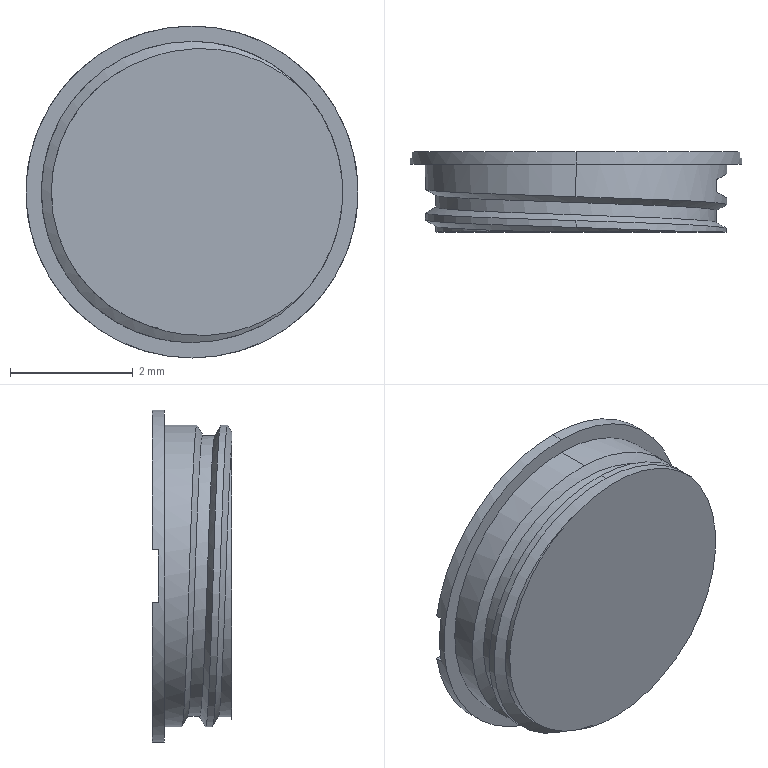Part | SolidWorks | features ICE 3, Extrusion 1, Helix 1, SweepCut 1 | 1 solid | 19 faces | box 5.4 x 1.3 x 5.4 mm | volume 23.765 mm3 | plane 10 | cylinder 6 | spline 3 | commonest cylinder face diameters 4.9 x4 5.4 x2
STEP:
#1=CARTESIAN_POINT('',(0.,1.3,2.7));
#2=VERTEX_POINT('',#1);
#3=CARTESIAN_POINT('',(2.666,1.3,0.425));
#4=VERTEX_POINT('',#3);
#5=CARTESIAN_POINT('',(0.,1.3,0.));
#6=DIRECTION('',(0.,1.,0.));
#7=DIRECTION('',(0.,0.,1.));
#8=AXIS2_PLACEMENT_3D('',#5,#6,#7);
#9=CIRCLE('',#8,2.7);
#10=EDGE_CURVE('',#2,#4,#9,.T.);
#11=ORIENTED_EDGE('',*,*,#10,.F.);
#12=CARTESIAN_POINT('',(0.,1.1,2.7));
#13=VERTEX_POINT('',#12);
#14=CARTESIAN_POINT('',(0.,1.3,2.7));
#15=DIRECTION('',(0.,-1.,0.));
#16=VECTOR('',#15,1000.);
#17=LINE('',#14,#16);
#18=EDGE_CURVE('',#2,#13,#17,.T.);
#19=ORIENTED_EDGE('',*,*,#18,.T.);
#20=CARTESIAN_POINT('',(0.,1.1,-2.7));
#21=VERTEX_POINT('',#20);
#22=CARTESIAN_POINT('',(0.,1.1,0.));
#23=DIRECTION('',(0.,-1.,0.));
#24=DIRECTION('',(0.,0.,-1.));
#25=AXIS2_PLACEMENT_3D('',#22,#23,#24);
#26=CIRCLE('',#25,2.7);
#27=EDGE_CURVE('',#21,#13,#26,.T.);
#28=ORIENTED_EDGE('',*,*,#27,.F.);
#29=CARTESIAN_POINT('',(0.,1.3,-2.7));
#30=VERTEX_POINT('',#29);
#31=CARTESIAN_POINT('',(0.,1.3,-2.7));
#32=DIRECTION('',(0.,-1.,0.));
#33=VECTOR('',#32,1000.);
#34=LINE('',#31,#33);
#35=EDGE_CURVE('',#30,#21,#34,.T.);
#36=ORIENTED_EDGE('',*,*,#35,.F.);
#37=CARTESIAN_POINT('',(2.666,1.3,-0.425));
#38=VERTEX_POINT('',#37);
#39=CARTESIAN_POINT('',(0.,1.3,0.));
#40=DIRECTION('',(0.,1.,0.));
#41=DIRECTION('',(0.,0.,1.));
#42=AXIS2_PLACEMENT_3D('',#39,#40,#41);
#43=CIRCLE('',#42,2.7);
#44=EDGE_CURVE('',#38,#30,#43,.T.);
#45=ORIENTED_EDGE('',*,*,#44,.F.);
#46=CARTESIAN_POINT('',(2.666,1.2,-0.425));
#47=VERTEX_POINT('',#46);
#48=CARTESIAN_POINT('',(2.666,1.3,-0.425));
#49=DIRECTION('',(0.,-1.,0.));
#50=VECTOR('',#49,1000.);
#51=LINE('',#48,#50);
#52=EDGE_CURVE('',#38,#47,#51,.T.);
#53=ORIENTED_EDGE('',*,*,#52,.T.);
#54=CARTESIAN_POINT('',(2.666,1.2,0.425));
#55=VERTEX_POINT('',#54);
#56=CARTESIAN_POINT('',(0.,1.2,0.));
#57=DIRECTION('',(0.,-1.,0.));
#58=DIRECTION('',(0.,0.,-1.));
#59=AXIS2_PLACEMENT_3D('',#56,#57,#58);
#60=CIRCLE('',#59,2.7);
#61=EDGE_CURVE('',#47,#55,#60,.T.);
#62=ORIENTED_EDGE('',*,*,#61,.T.);
#63=CARTESIAN_POINT('',(2.666,1.3,0.425));
#64=DIRECTION('',(0.,1.,0.));
#65=VECTOR('',#64,1000.);
#66=LINE('',#63,#65);
#67=EDGE_CURVE('',#55,#4,#66,.T.);
#68=ORIENTED_EDGE('',*,*,#67,.T.);
#69=EDGE_LOOP('',(#11,#19,#28,#36,#45,#53,#62,#68));
#70=FACE_OUTER_BOUND('',#69,.T.);
#71=CARTESIAN_POINT('',(0.,1.3,0.));
#72=DIRECTION('',(0.,-1.,0.));
#73=DIRECTION('',(0.,0.,-1.));
#74=AXIS2_PLACEMENT_3D('',#71,#72,#73);
#75=CYLINDRICAL_SURFACE('',#74,2.7);
#76=ADVANCED_FACE('',(#70),#75,.T.);
#77=CARTESIAN_POINT('',(0.,1.1,-2.45));
#78=VERTEX_POINT('',#77);
#79=CARTESIAN_POINT('',(0.,1.1,2.45));
#80=VERTEX_POINT('',#79);
#81=CARTESIAN_POINT('',(0.,1.1,0.));
#82=DIRECTION('',(0.,-1.,0.));
#83=DIRECTION('',(0.,0.,-1.));
#84=AXIS2_PLACEMENT_3D('',#81,#82,#83);
#85=CIRCLE('',#84,2.45);
#86=EDGE_CURVE('',#78,#80,#85,.T.);
#87=ORIENTED_EDGE('',*,*,#86,.T.);
#88=CARTESIAN_POINT('',(0.,0.5692,2.45));
#89=VERTEX_POINT('',#88);
#90=CARTESIAN_POINT('',(0.,1.1,2.45));
#91=DIRECTION('',(0.,-1.,0.));
#92=VECTOR('',#91,1000.);
#93=LINE('',#90,#92);
#94=EDGE_CURVE('',#80,#89,#93,.T.);
#95=ORIENTED_EDGE('',*,*,#94,.T.);
#96=CARTESIAN_POINT('',(0.,0.3192,-2.45));
#97=VERTEX_POINT('',#96);
#98=CARTESIAN_POINT('',(0.,0.3192,-2.45));
#99=CARTESIAN_POINT('',(0.6565,0.3416,-2.45));
#100=CARTESIAN_POINT('',(1.225,0.3609,-2.122));
#101=CARTESIAN_POINT('',(2.45,0.4026,-1.415));
#102=CARTESIAN_POINT('',(2.45,0.4442,0.));
#103=CARTESIAN_POINT('',(2.45,0.4859,1.415));
#104=CARTESIAN_POINT('',(1.225,0.5276,2.122));
#105=CARTESIAN_POINT('',(0.6565,0.5469,2.45));
#106=CARTESIAN_POINT('',(0.,0.5692,2.45));
#107=(BOUNDED_CURVE()B_SPLINE_CURVE(2,(#98,#99,#100,#101,#102,#103,#104,#105,#106),.UNSPECIFIED.,.F.,.F.)B_SPLINE_CURVE_WITH_KNOTS((3,2,2,2,3),(0.4167,0.4444,0.5,0.5556,0.5833),.UNSPECIFIED.)CURVE()GEOMETRIC_REPRESENTATION_ITEM()RATIONAL_B_SPLINE_CURVE((0.933,0.933,1.,0.866,1.,0.866,1.,0.933,0.933))REPRESENTATION_ITEM(''));
#108=EDGE_CURVE('',#97,#89,#107,.T.);
#109=ORIENTED_EDGE('',*,*,#108,.F.);
#110=CARTESIAN_POINT('',(0.,0.4308,-2.45));
#111=VERTEX_POINT('',#110);
#112=CARTESIAN_POINT('',(0.,1.1,-2.45));
#113=DIRECTION('',(0.,-1.,0.));
#114=VECTOR('',#113,1000.);
#115=LINE('',#112,#114);
#116=EDGE_CURVE('',#111,#97,#115,.T.);
#117=ORIENTED_EDGE('',*,*,#116,.F.);
#118=CARTESIAN_POINT('',(2.45,0.5558,0.));
#119=VERTEX_POINT('',#118);
#120=CARTESIAN_POINT('',(0.,0.4308,-2.45));
#121=CARTESIAN_POINT('',(0.6565,0.4531,-2.45));
#122=CARTESIAN_POINT('',(1.225,0.4724,-2.122));
#123=CARTESIAN_POINT('',(2.45,0.5141,-1.415));
#124=CARTESIAN_POINT('',(2.45,0.5558,0.));
#125=(BOUNDED_CURVE()B_SPLINE_CURVE(2,(#120,#121,#122,#123,#124),.UNSPECIFIED.,.F.,.F.)B_SPLINE_CURVE_WITH_KNOTS((3,2,3),(0.75,0.7778,0.8333),.UNSPECIFIED.)CURVE()GEOMETRIC_REPRESENTATION_ITEM()RATIONAL_B_SPLINE_CURVE((0.933,0.933,1.,0.866,1.))REPRESENTATION_ITEM(''));
#126=EDGE_CURVE('',#111,#119,#125,.T.);
#127=ORIENTED_EDGE('',*,*,#126,.T.);
#128=CARTESIAN_POINT('',(2.287,0.65,0.8792));
#129=VERTEX_POINT('',#128);
#130=CARTESIAN_POINT('',(2.287,0.65,0.8792));
#131=CARTESIAN_POINT('',(2.395,0.5875,0.5979));
#132=CARTESIAN_POINT('',(2.45,0.5558,0.3015));
#133=CARTESIAN_POINT('',(2.45,0.5558,0.));
#134=(BOUNDED_CURVE()B_SPLINE_CURVE(3,(#130,#131,#132,#133),.UNSPECIFIED.,.F.,.F.)B_SPLINE_CURVE_WITH_KNOTS((4,4),(5.916,6.283),.UNSPECIFIED.)CURVE()GEOMETRIC_REPRESENTATION_ITEM()RATIONAL_B_SPLINE_CURVE((1.,0.9888,0.9888,1.))REPRESENTATION_ITEM(''));
#135=EDGE_CURVE('',#129,#119,#134,.T.);
#136=ORIENTED_EDGE('',*,*,#135,.F.);
#137=CARTESIAN_POINT('',(2.287,0.85,0.8792));
#138=VERTEX_POINT('',#137);
#139=CARTESIAN_POINT('',(2.287,1.1,0.8792));
#140=DIRECTION('',(0.,-1.,0.));
#141=VECTOR('',#140,1000.);
#142=LINE('',#139,#141);
#143=EDGE_CURVE('',#138,#129,#142,.T.);
#144=ORIENTED_EDGE('',*,*,#143,.F.);
#145=CARTESIAN_POINT('',(2.45,0.9442,0.));
#146=VERTEX_POINT('',#145);
#147=CARTESIAN_POINT('',(2.45,0.9442,0.));
#148=CARTESIAN_POINT('',(2.45,0.9442,0.3015));
#149=CARTESIAN_POINT('',(2.395,0.9125,0.5979));
#150=CARTESIAN_POINT('',(2.287,0.85,0.8792));
#151=(BOUNDED_CURVE()B_SPLINE_CURVE(3,(#147,#148,#149,#150),.UNSPECIFIED.,.F.,.F.)B_SPLINE_CURVE_WITH_KNOTS((4,4),(3.142,3.509),.UNSPECIFIED.)CURVE()GEOMETRIC_REPRESENTATION_ITEM()RATIONAL_B_SPLINE_CURVE((1.,0.9888,0.9888,1.))REPRESENTATION_ITEM(''));
#152=EDGE_CURVE('',#146,#138,#151,.T.);
#153=ORIENTED_EDGE('',*,*,#152,.F.);
#154=CARTESIAN_POINT('',(0.,0.8192,-2.45));
#155=VERTEX_POINT('',#154);
#156=CARTESIAN_POINT('',(0.,0.8192,-2.45));
#157=CARTESIAN_POINT('',(0.6565,0.8416,-2.45));
#158=CARTESIAN_POINT('',(1.225,0.8609,-2.122));
#159=CARTESIAN_POINT('',(2.45,0.9026,-1.415));
#160=CARTESIAN_POINT('',(2.45,0.9442,0.));
#161=(BOUNDED_CURVE()B_SPLINE_CURVE(2,(#156,#157,#158,#159,#160),.UNSPECIFIED.,.F.,.F.)B_SPLINE_CURVE_WITH_KNOTS((3,2,3),(0.75,0.7778,0.8333),.UNSPECIFIED.)CURVE()GEOMETRIC_REPRESENTATION_ITEM()RATIONAL_B_SPLINE_CURVE((0.933,0.933,1.,0.866,1.))REPRESENTATION_ITEM(''));
#162=EDGE_CURVE('',#155,#146,#161,.T.);
#163=ORIENTED_EDGE('',*,*,#162,.F.);
#164=CARTESIAN_POINT('',(0.,1.1,-2.45));
#165=DIRECTION('',(0.,-1.,0.));
#166=VECTOR('',#165,1000.);
#167=LINE('',#164,#166);
#168=EDGE_CURVE('',#78,#155,#167,.T.);
#169=ORIENTED_EDGE('',*,*,#168,.F.);
#170=EDGE_LOOP('',(#87,#95,#109,#117,#127,#136,#144,#153,#163,#169));
#171=FACE_OUTER_BOUND('',#170,.T.);
#172=CARTESIAN_POINT('',(0.,1.1,0.));
#173=DIRECTION('',(0.,-1.,0.));
#174=DIRECTION('',(0.,0.,-1.));
#175=AXIS2_PLACEMENT_3D('',#172,#173,#174);
#176=CYLINDRICAL_SURFACE('',#175,2.45);
#177=ADVANCED_FACE('',(#171),#176,.T.);
#178=CARTESIAN_POINT('',(1.884,0.,-1.566));
#179=VERTEX_POINT('',#178);
#180=CARTESIAN_POINT('',(0.,0.1808,2.45));
#181=VERTEX_POINT('',#180);
#182=CARTESIAN_POINT('',(1.884,0.,-1.566));
#183=CARTESIAN_POINT('',(2.45,0.02969,-0.8856));
#184=CARTESIAN_POINT('',(2.45,0.05577,0.));
#185=CARTESIAN_POINT('',(2.45,0.09744,1.415));
#186=CARTESIAN_POINT('',(1.225,0.1391,2.122));
#187=CARTESIAN_POINT('',(0.6565,0.1584,2.45));
#188=CARTESIAN_POINT('',(0.,0.1808,2.45));
#189=(BOUNDED_CURVE()B_SPLINE_CURVE(2,(#182,#183,#184,#185,#186,#187,#188),.UNSPECIFIED.,.F.,.F.)B_SPLINE_CURVE_WITH_KNOTS((3,2,2,3),(0.4634,0.5,0.5556,0.5833),.UNSPECIFIED.)CURVE()GEOMETRIC_REPRESENTATION_ITEM()RATIONAL_B_SPLINE_CURVE((0.9398,0.9117,1.,0.866,1.,0.933,0.933))REPRESENTATION_ITEM(''));
#190=EDGE_CURVE('',#179,#181,#189,.T.);
#191=ORIENTED_EDGE('',*,*,#190,.T.);
#192=CARTESIAN_POINT('',(0.,0.06923,2.45));
#193=VERTEX_POINT('',#192);
#194=CARTESIAN_POINT('',(0.,1.1,2.45));
#195=DIRECTION('',(0.,-1.,0.));
#196=VECTOR('',#195,1000.);
#197=LINE('',#194,#196);
#198=EDGE_CURVE('',#181,#193,#197,.T.);
#199=ORIENTED_EDGE('',*,*,#198,.T.);
#200=CARTESIAN_POINT('',(1.884,0.,1.566));
#201=VERTEX_POINT('',#200);
#202=CARTESIAN_POINT('',(1.884,0.,1.566));
#203=CARTESIAN_POINT('',(1.604,0.01467,1.903));
#204=CARTESIAN_POINT('',(1.225,0.02756,2.122));
#205=CARTESIAN_POINT('',(0.6565,0.0469,2.45));
#206=CARTESIAN_POINT('',(0.,0.06923,2.45));
#207=(BOUNDED_CURVE()B_SPLINE_CURVE(2,(#202,#203,#204,#205,#206),.UNSPECIFIED.,.F.,.F.)B_SPLINE_CURVE_WITH_KNOTS((3,2,3),(0.2033,0.2222,0.25),.UNSPECIFIED.)CURVE()GEOMETRIC_REPRESENTATION_ITEM()RATIONAL_B_SPLINE_CURVE((0.9398,0.9543,1.,0.933,0.933))REPRESENTATION_ITEM(''));
#208=EDGE_CURVE('',#201,#193,#207,.T.);
#209=ORIENTED_EDGE('',*,*,#208,.F.);
#210=CARTESIAN_POINT('',(0.,0.,0.));
#211=DIRECTION('',(0.,-1.,0.));
#212=DIRECTION('',(0.,0.,-1.));
#213=AXIS2_PLACEMENT_3D('',#210,#211,#212);
#214=CIRCLE('',#213,2.45);
#215=EDGE_CURVE('',#179,#201,#214,.T.);
#216=ORIENTED_EDGE('',*,*,#215,.F.);
#217=EDGE_LOOP('',(#191,#199,#209,#216));
#218=FACE_OUTER_BOUND('',#217,.T.);
#219=CARTESIAN_POINT('',(0.,1.1,0.));
#220=DIRECTION('',(0.,-1.,0.));
#221=DIRECTION('',(0.,0.,-1.));
#222=AXIS2_PLACEMENT_3D('',#219,#220,#221);
#223=CYLINDRICAL_SURFACE('',#222,2.45);
#224=ADVANCED_FACE('',(#218),#223,.T.);
#225=ORIENTED_EDGE('',*,*,#198,.F.);
#226=CARTESIAN_POINT('',(0.,0.1808,2.45));
#227=CARTESIAN_POINT('',(-0.6565,0.2031,2.45));
#228=CARTESIAN_POINT('',(-1.225,0.2224,2.122));
#229=CARTESIAN_POINT('',(-2.45,0.2641,1.415));
#230=CARTESIAN_POINT('',(-2.45,0.3058,0.));
#231=CARTESIAN_POINT('',(-2.45,0.3474,-1.415));
#232=CARTESIAN_POINT('',(-1.225,0.3891,-2.122));
#233=CARTESIAN_POINT('',(-0.6565,0.4084,-2.45));
#234=CARTESIAN_POINT('',(0.,0.4308,-2.45));
#235=(BOUNDED_CURVE()B_SPLINE_CURVE(2,(#226,#227,#228,#229,#230,#231,#232,#233,#234),.UNSPECIFIED.,.F.,.F.)B_SPLINE_CURVE_WITH_KNOTS((3,2,2,2,3),(0.5833,0.6111,0.6667,0.7222,0.75),.UNSPECIFIED.)CURVE()GEOMETRIC_REPRESENTATION_ITEM()RATIONAL_B_SPLINE_CURVE((0.933,0.933,1.,0.866,1.,0.866,1.,0.933,0.933))REPRESENTATION_ITEM(''));
#236=EDGE_CURVE('',#181,#111,#235,.T.);
#237=ORIENTED_EDGE('',*,*,#236,.T.);
#238=ORIENTED_EDGE('',*,*,#116,.T.);
#239=CARTESIAN_POINT('',(0.,0.06923,2.45));
#240=CARTESIAN_POINT('',(-0.6565,0.09156,2.45));
#241=CARTESIAN_POINT('',(-1.225,0.1109,2.122));
#242=CARTESIAN_POINT('',(-2.45,0.1526,1.415));
#243=CARTESIAN_POINT('',(-2.45,0.1942,0.));
#244=CARTESIAN_POINT('',(-2.45,0.2359,-1.415));
#245=CARTESIAN_POINT('',(-1.225,0.2776,-2.122));
#246=CARTESIAN_POINT('',(-0.6565,0.2969,-2.45));
#247=CARTESIAN_POINT('',(0.,0.3192,-2.45));
#248=(BOUNDED_CURVE()B_SPLINE_CURVE(2,(#239,#240,#241,#242,#243,#244,#245,#246,#247),.UNSPECIFIED.,.F.,.F.)B_SPLINE_CURVE_WITH_KNOTS((3,2,2,2,3),(0.25,0.2778,0.3333,0.3889,0.4167),.UNSPECIFIED.)CURVE()GEOMETRIC_REPRESENTATION_ITEM()RATIONAL_B_SPLINE_CURVE((0.933,0.933,1.,0.866,1.,0.866,1.,0.933,0.933))REPRESENTATION_ITEM(''));
#249=EDGE_CURVE('',#193,#97,#248,.T.);
#250=ORIENTED_EDGE('',*,*,#249,.F.);
#251=EDGE_LOOP('',(#225,#237,#238,#250));
#252=FACE_OUTER_BOUND('',#251,.T.);
#253=CARTESIAN_POINT('',(0.,1.1,0.));
#254=DIRECTION('',(0.,-1.,0.));
#255=DIRECTION('',(0.,0.,-1.));
#256=AXIS2_PLACEMENT_3D('',#253,#254,#255);
#257=CYLINDRICAL_SURFACE('',#256,2.45);
#258=ADVANCED_FACE('',(#252),#257,.T.);
#259=CARTESIAN_POINT('',(-2.666,1.3,0.425));
#260=VERTEX_POINT('',#259);
#261=CARTESIAN_POINT('',(0.,1.3,0.425));
#262=DIRECTION('',(1.,0.,0.));
#263=VECTOR('',#262,1000.);
#264=LINE('',#261,#263);
#265=EDGE_CURVE('',#260,#4,#264,.T.);
#266=ORIENTED_EDGE('',*,*,#265,.F.);
#267=CARTESIAN_POINT('',(0.,1.3,0.));
#268=DIRECTION('',(0.,1.,0.));
#269=DIRECTION('',(0.,0.,1.));
#270=AXIS2_PLACEMENT_3D('',#267,#268,#269);
#271=CIRCLE('',#270,2.7);
#272=EDGE_CURVE('',#260,#2,#271,.T.);
#273=ORIENTED_EDGE('',*,*,#272,.T.);
#274=ORIENTED_EDGE('',*,*,#10,.T.);
#275=EDGE_LOOP('',(#266,#273,#274));
#276=FACE_OUTER_BOUND('',#275,.T.);
#277=CARTESIAN_POINT('',(0.,1.3,0.));
#278=DIRECTION('',(0.,1.,0.));
#279=DIRECTION('',(0.,0.,1.));
#280=AXIS2_PLACEMENT_3D('',#277,#278,#279);
#281=PLANE('',#280);
#282=ADVANCED_FACE('',(#276),#281,.T.);
#283=ORIENTED_EDGE('',*,*,#94,.F.);
#284=CARTESIAN_POINT('',(0.,1.1,0.));
#285=DIRECTION('',(0.,-1.,0.));
#286=DIRECTION('',(0.,0.,-1.));
#287=AXIS2_PLACEMENT_3D('',#284,#285,#286);
#288=CIRCLE('',#287,2.45);
#289=EDGE_CURVE('',#80,#78,#288,.T.);
#290=ORIENTED_EDGE('',*,*,#289,.T.);
#291=ORIENTED_EDGE('',*,*,#168,.T.);
#292=CARTESIAN_POINT('',(0.,0.5692,2.45));
#293=CARTESIAN_POINT('',(-0.6565,0.5916,2.45));
#294=CARTESIAN_POINT('',(-1.225,0.6109,2.122));
#295=CARTESIAN_POINT('',(-2.45,0.6526,1.415));
#296=CARTESIAN_POINT('',(-2.45,0.6942,0.));
#297=CARTESIAN_POINT('',(-2.45,0.7359,-1.415));
#298=CARTESIAN_POINT('',(-1.225,0.7776,-2.122));
#299=CARTESIAN_POINT('',(-0.6565,0.7969,-2.45));
#300=CARTESIAN_POINT('',(0.,0.8192,-2.45));
#301=(BOUNDED_CURVE()B_SPLINE_CURVE(2,(#292,#293,#294,#295,#296,#297,#298,#299,#300),.UNSPECIFIED.,.F.,.F.)B_SPLINE_CURVE_WITH_KNOTS((3,2,2,2,3),(0.5833,0.6111,0.6667,0.7222,0.75),.UNSPECIFIED.)CURVE()GEOMETRIC_REPRESENTATION_ITEM()RATIONAL_B_SPLINE_CURVE((0.933,0.933,1.,0.866,1.,0.866,1.,0.933,0.933))REPRESENTATION_ITEM(''));
#302=EDGE_CURVE('',#89,#155,#301,.T.);
#303=ORIENTED_EDGE('',*,*,#302,.F.);
#304=EDGE_LOOP('',(#283,#290,#291,#303));
#305=FACE_OUTER_BOUND('',#304,.T.);
#306=CARTESIAN_POINT('',(0.,1.1,0.));
#307=DIRECTION('',(0.,-1.,0.));
#308=DIRECTION('',(0.,0.,-1.));
#309=AXIS2_PLACEMENT_3D('',#306,#307,#308);
#310=CYLINDRICAL_SURFACE('',#309,2.45);
#311=ADVANCED_FACE('',(#305),#310,.T.);
#312=CARTESIAN_POINT('',(-0.686,0.,-2.181));
#313=VERTEX_POINT('',#312);
#314=CARTESIAN_POINT('',(1.884,0.,-1.566));
#315=CARTESIAN_POINT('',(1.723,0.,-1.738));
#316=CARTESIAN_POINT('',(1.538,0.,-1.887));
#317=CARTESIAN_POINT('',(1.138,0.,-2.124));
#318=CARTESIAN_POINT('',(0.9167,0.,-2.215));
#319=CARTESIAN_POINT('',(0.5773,0.,-2.297));
#320=CARTESIAN_POINT('',(0.4626,0.,-2.316));
#321=CARTESIAN_POINT('',(0.2298,0.,-2.336));
#322=CARTESIAN_POINT('',(0.111,0.,-2.337));
#323=CARTESIAN_POINT('',(-0.2385,0.,-2.315));
#324=CARTESIAN_POINT('',(-0.4654,0.,-2.266));
#325=CARTESIAN_POINT('',(-0.686,0.,-2.181));
#326=B_SPLINE_CURVE_WITH_KNOTS('',3,(#314,#315,#316,#317,#318,#319,#320,#321,#322,#323,#324,#325),.UNSPECIFIED.,.F.,.F.,(4,2,2,2,2,4),(0.0001717,0.0008766,0.001582,0.001934,0.002286,0.002991),.UNSPECIFIED.);
#327=EDGE_CURVE('',#179,#313,#326,.T.);
#328=ORIENTED_EDGE('',*,*,#327,.F.);
#329=ORIENTED_EDGE('',*,*,#215,.T.);
#330=CARTESIAN_POINT('',(-0.686,0.,2.181));
#331=VERTEX_POINT('',#330);
#332=CARTESIAN_POINT('',(-0.686,0.,2.181));
#333=CARTESIAN_POINT('',(-0.2463,0.,2.349));
#334=CARTESIAN_POINT('',(0.237,0.,2.38));
#335=CARTESIAN_POINT('',(1.149,0.,2.158));
#336=CARTESIAN_POINT('',(1.564,0.,1.908));
#337=CARTESIAN_POINT('',(1.884,0.,1.566));
#338=B_SPLINE_CURVE_WITH_KNOTS('',3,(#332,#333,#334,#335,#336,#337),.UNSPECIFIED.,.F.,.F.,(4,2,4),(0.,0.001406,0.002811),.UNSPECIFIED.);
#339=EDGE_CURVE('',#331,#201,#338,.T.);
#340=ORIENTED_EDGE('',*,*,#339,.F.);
#341=CARTESIAN_POINT('',(-0.686,0.,-2.181));
#342=CARTESIAN_POINT('',(-0.9183,0.,-2.108));
#343=CARTESIAN_POINT('',(-1.138,0.,-1.998));
#344=CARTESIAN_POINT('',(-1.528,0.,-1.718));
#345=CARTESIAN_POINT('',(-1.703,0.,-1.545));
#346=CARTESIAN_POINT('',(-1.916,0.,-1.254));
#347=CARTESIAN_POINT('',(-1.979,0.,-1.152));
#348=CARTESIAN_POINT('',(-2.09,0.,-0.937));
#349=CARTESIAN_POINT('',(-2.137,0.,-0.824));
#350=CARTESIAN_POINT('',(-2.211,0.,-0.5953));
#351=CARTESIAN_POINT('',(-2.239,0.,-0.4786));
#352=CARTESIAN_POINT('',(-2.277,0.,-0.2407));
#353=CARTESIAN_POINT('',(-2.287,0.,-0.1185));
#354=CARTESIAN_POINT('',(-2.287,0.,0.1225));
#355=CARTESIAN_POINT('',(-2.277,0.,0.2421));
#356=CARTESIAN_POINT('',(-2.239,0.,0.4797));
#357=CARTESIAN_POINT('',(-2.21,0.,0.5986));
#358=CARTESIAN_POINT('',(-2.097,0.,0.9428));
#359=CARTESIAN_POINT('',(-1.986,0.,1.159));
#360=CARTESIAN_POINT('',(-1.7,0.,1.549));
#361=CARTESIAN_POINT('',(-1.528,0.,1.719));
#362=CARTESIAN_POINT('',(-1.133,0.,2.001));
#363=CARTESIAN_POINT('',(-0.9183,0.,2.108));
#364=CARTESIAN_POINT('',(-0.686,0.,2.181));
#365=B_SPLINE_CURVE_WITH_KNOTS('',3,(#341,#342,#343,#344,#345,#346,#347,#348,#349,#350,#351,#352,#353,#354,#355,#356,#357,#358,#359,#360,#361,#362,#363,#364),.UNSPECIFIED.,.F.,.F.,(4,2,2,2,2,2,2,2,2,2,2,4),(0.,0.0007276,0.001455,0.001819,0.002183,0.002547,0.00291,0.003274,0.003638,0.004365,0.005093,0.005821),.UNSPECIFIED.);
#366=EDGE_CURVE('',#313,#331,#365,.T.);
#367=ORIENTED_EDGE('',*,*,#366,.F.);
#368=EDGE_LOOP('',(#328,#329,#340,#367));
#369=FACE_OUTER_BOUND('',#368,.T.);
#370=CARTESIAN_POINT('',(0.,0.,0.));
#371=DIRECTION('',(0.,1.,0.));
#372=DIRECTION('',(0.,0.,1.));
#373=AXIS2_PLACEMENT_3D('',#370,#371,#372);
#374=PLANE('',#373);
#375=ADVANCED_FACE('',(#369),#374,.F.);
#376=ORIENTED_EDGE('',*,*,#18,.F.);
#377=ORIENTED_EDGE('',*,*,#272,.F.);
#378=CARTESIAN_POINT('',(-2.666,1.2,0.425));
#379=VERTEX_POINT('',#378);
#380=CARTESIAN_POINT('',(-2.666,1.3,0.425));
#381=DIRECTION('',(0.,-1.,0.));
#382=VECTOR('',#381,1000.);
#383=LINE('',#380,#382);
#384=EDGE_CURVE('',#260,#379,#383,.T.);
#385=ORIENTED_EDGE('',*,*,#384,.T.);
#386=CARTESIAN_POINT('',(-2.666,1.2,-0.425));
#387=VERTEX_POINT('',#386);
#388=CARTESIAN_POINT('',(0.,1.2,0.));
#389=DIRECTION('',(0.,-1.,0.));
#390=DIRECTION('',(0.,0.,-1.));
#391=AXIS2_PLACEMENT_3D('',#388,#389,#390);
#392=CIRCLE('',#391,2.7);
#393=EDGE_CURVE('',#379,#387,#392,.T.);
#394=ORIENTED_EDGE('',*,*,#393,.T.);
#395=CARTESIAN_POINT('',(-2.666,1.3,-0.425));
#396=VERTEX_POINT('',#395);
#397=CARTESIAN_POINT('',(-2.666,1.3,-0.425));
#398=DIRECTION('',(0.,1.,0.));
#399=VECTOR('',#398,1000.);
#400=LINE('',#397,#399);
#401=EDGE_CURVE('',#387,#396,#400,.T.);
#402=ORIENTED_EDGE('',*,*,#401,.T.);
#403=CARTESIAN_POINT('',(0.,1.3,0.));
#404=DIRECTION('',(0.,1.,0.));
#405=DIRECTION('',(0.,0.,1.));
#406=AXIS2_PLACEMENT_3D('',#403,#404,#405);
#407=CIRCLE('',#406,2.7);
#408=EDGE_CURVE('',#30,#396,#407,.T.);
#409=ORIENTED_EDGE('',*,*,#408,.F.);
#410=ORIENTED_EDGE('',*,*,#35,.T.);
#411=CARTESIAN_POINT('',(0.,1.1,0.));
#412=DIRECTION('',(0.,-1.,0.));
#413=DIRECTION('',(0.,0.,-1.));
#414=AXIS2_PLACEMENT_3D('',#411,#412,#413);
#415=CIRCLE('',#414,2.7);
#416=EDGE_CURVE('',#13,#21,#415,.T.);
#417=ORIENTED_EDGE('',*,*,#416,.F.);
#418=EDGE_LOOP('',(#376,#377,#385,#394,#402,#409,#410,#417));
#419=FACE_OUTER_BOUND('',#418,.T.);
#420=CARTESIAN_POINT('',(0.,1.3,0.));
#421=DIRECTION('',(0.,-1.,0.));
#422=DIRECTION('',(0.,0.,-1.));
#423=AXIS2_PLACEMENT_3D('',#420,#421,#422);
#424=CYLINDRICAL_SURFACE('',#423,2.7);
#425=ADVANCED_FACE('',(#419),#424,.T.);
#426=CARTESIAN_POINT('',(0.,1.3,-0.425));
#427=DIRECTION('',(-1.,0.,0.));
#428=VECTOR('',#427,1000.);
#429=LINE('',#426,#428);
#430=EDGE_CURVE('',#38,#396,#429,.T.);
#431=ORIENTED_EDGE('',*,*,#430,.F.);
#432=ORIENTED_EDGE('',*,*,#44,.T.);
#433=ORIENTED_EDGE('',*,*,#408,.T.);
#434=EDGE_LOOP('',(#431,#432,#433));
#435=FACE_OUTER_BOUND('',#434,.T.);
#436=CARTESIAN_POINT('',(0.,1.3,0.));
#437=DIRECTION('',(0.,1.,0.));
#438=DIRECTION('',(0.,0.,1.));
#439=AXIS2_PLACEMENT_3D('',#436,#437,#438);
#440=PLANE('',#439);
#441=ADVANCED_FACE('',(#435),#440,.T.);
#442=ORIENTED_EDGE('',*,*,#86,.F.);
#443=ORIENTED_EDGE('',*,*,#289,.F.);
#444=EDGE_LOOP('',(#442,#443));
#445=FACE_BOUND('',#444,.T.);
#446=ORIENTED_EDGE('',*,*,#27,.T.);
#447=ORIENTED_EDGE('',*,*,#416,.T.);
#448=EDGE_LOOP('',(#446,#447));
#449=FACE_OUTER_BOUND('',#448,.T.);
#450=CARTESIAN_POINT('',(0.,1.1,0.));
#451=DIRECTION('',(0.,-1.,0.));
#452=DIRECTION('',(0.,0.,-1.));
#453=AXIS2_PLACEMENT_3D('',#450,#451,#452);
#454=PLANE('',#453);
#455=ADVANCED_FACE('',(#445,#449),#454,.T.);
#456=ORIENTED_EDGE('',*,*,#208,.T.);
#457=ORIENTED_EDGE('',*,*,#249,.T.);
#458=ORIENTED_EDGE('',*,*,#108,.T.);
#459=ORIENTED_EDGE('',*,*,#302,.T.);
#460=ORIENTED_EDGE('',*,*,#162,.T.);
#461=CARTESIAN_POINT('',(2.287,0.85,0.));
#462=VERTEX_POINT('',#461);
#463=CARTESIAN_POINT('',(2.287,0.85,0.));
#464=CARTESIAN_POINT('',(2.341,0.8814,0.));
#465=CARTESIAN_POINT('',(2.396,0.9128,0.));
#466=CARTESIAN_POINT('',(2.45,0.9442,0.));
#467=B_SPLINE_CURVE_WITH_KNOTS('',3,(#463,#464,#465,#466),.UNSPECIFIED.,.F.,.F.,(4,4),(0.,1.),.UNSPECIFIED.);
#468=EDGE_CURVE('',#462,#146,#467,.T.);
#469=ORIENTED_EDGE('',*,*,#468,.F.);
#470=CARTESIAN_POINT('',(-0.686,0.,2.181));
#471=CARTESIAN_POINT('',(-0.9258,0.008736,2.106));
#472=CARTESIAN_POINT('',(-1.143,0.01667,1.98));
#473=CARTESIAN_POINT('',(-2.287,0.05833,1.32));
#474=CARTESIAN_POINT('',(-2.287,0.1,0.));
#475=CARTESIAN_POINT('',(-2.287,0.1417,-1.32));
#476=CARTESIAN_POINT('',(-1.143,0.1833,-1.98));
#477=CARTESIAN_POINT('',(0.,0.225,-2.641));
#478=CARTESIAN_POINT('',(1.143,0.2667,-1.98));
#479=CARTESIAN_POINT('',(2.287,0.3083,-1.32));
#480=CARTESIAN_POINT('',(2.287,0.35,0.));
#481=CARTESIAN_POINT('',(2.287,0.3917,1.32));
#482=CARTESIAN_POINT('',(1.143,0.4333,1.98));
#483=CARTESIAN_POINT('',(0.,0.475,2.641));
#484=CARTESIAN_POINT('',(-1.143,0.5167,1.98));
#485=CARTESIAN_POINT('',(-2.287,0.5583,1.32));
#486=CARTESIAN_POINT('',(-2.287,0.6,0.));
#487=CARTESIAN_POINT('',(-2.287,0.6417,-1.32));
#488=CARTESIAN_POINT('',(-1.143,0.6833,-1.98));
#489=CARTESIAN_POINT('',(0.,0.725,-2.641));
#490=CARTESIAN_POINT('',(1.143,0.7667,-1.98));
#491=CARTESIAN_POINT('',(2.287,0.8083,-1.32));
#492=CARTESIAN_POINT('',(2.287,0.85,0.));
#493=(BOUNDED_CURVE()B_SPLINE_CURVE(2,(#470,#471,#472,#473,#474,#475,#476,#477,#478,#479,#480,#481,#482,#483,#484,#485,#486,#487,#488,#489,#490,#491,#492),.UNSPECIFIED.,.F.,.F.)B_SPLINE_CURVE_WITH_KNOTS((3,2,2,2,2,2,2,2,2,2,2,3),(0.2659,0.2778,0.3333,0.3889,0.4444,0.5,0.5556,0.6111,0.6667,0.7222,0.7778,0.8333),.UNSPECIFIED.)CURVE()GEOMETRIC_REPRESENTATION_ITEM()RATIONAL_B_SPLINE_CURVE((0.955,0.9714,1.,0.866,1.,0.866,1.,0.866,1.,0.866,1.,0.866,1.,0.866,1.,0.866,1.,0.866,1.,0.866,1.,0.866,1.))REPRESENTATION_ITEM(''));
#494=EDGE_CURVE('',#331,#462,#493,.T.);
#495=ORIENTED_EDGE('',*,*,#494,.F.);
#496=ORIENTED_EDGE('',*,*,#339,.T.);
#497=EDGE_LOOP('',(#456,#457,#458,#459,#460,#469,#495,#496));
#498=FACE_OUTER_BOUND('',#497,.T.);
#499=CARTESIAN_POINT('',(-2.287,-0.4,0.));
#500=CARTESIAN_POINT('',(-2.287,-0.3583,-1.32));
#501=CARTESIAN_POINT('',(-1.143,-0.3167,-1.98));
#502=CARTESIAN_POINT('',(0.,-0.275,-2.641));
#503=CARTESIAN_POINT('',(1.143,-0.2333,-1.98));
#504=CARTESIAN_POINT('',(2.287,-0.1917,-1.32));
#505=CARTESIAN_POINT('',(2.287,-0.15,0.));
#506=CARTESIAN_POINT('',(2.287,-0.1083,1.32));
#507=CARTESIAN_POINT('',(1.143,-0.06667,1.98));
#508=CARTESIAN_POINT('',(0.,-0.025,2.641));
#509=CARTESIAN_POINT('',(-1.143,0.01667,1.98));
#510=CARTESIAN_POINT('',(-2.287,0.05833,1.32));
#511=CARTESIAN_POINT('',(-2.287,0.1,0.));
#512=CARTESIAN_POINT('',(-2.287,0.1417,-1.32));
#513=CARTESIAN_POINT('',(-1.143,0.1833,-1.98));
#514=CARTESIAN_POINT('',(0.,0.225,-2.641));
#515=CARTESIAN_POINT('',(1.143,0.2667,-1.98));
#516=CARTESIAN_POINT('',(2.287,0.3083,-1.32));
#517=CARTESIAN_POINT('',(2.287,0.35,0.));
#518=CARTESIAN_POINT('',(2.287,0.3917,1.32));
#519=CARTESIAN_POINT('',(1.143,0.4333,1.98));
#520=CARTESIAN_POINT('',(0.,0.475,2.641));
#521=CARTESIAN_POINT('',(-1.143,0.5167,1.98));
#522=CARTESIAN_POINT('',(-2.287,0.5583,1.32));
#523=CARTESIAN_POINT('',(-2.287,0.6,0.));
#524=CARTESIAN_POINT('',(-2.287,0.6417,-1.32));
#525=CARTESIAN_POINT('',(-1.143,0.6833,-1.98));
#526=CARTESIAN_POINT('',(0.,0.725,-2.641));
#527=CARTESIAN_POINT('',(1.143,0.7667,-1.98));
#528=CARTESIAN_POINT('',(2.287,0.8083,-1.32));
#529=CARTESIAN_POINT('',(2.287,0.85,0.));
#530=CARTESIAN_POINT('',(-2.46,-0.3,0.));
#531=CARTESIAN_POINT('',(-2.46,-0.2583,-1.42));
#532=CARTESIAN_POINT('',(-1.23,-0.2167,-2.13));
#533=CARTESIAN_POINT('',(0.,-0.175,-2.841));
#534=CARTESIAN_POINT('',(1.23,-0.1333,-2.13));
#535=CARTESIAN_POINT('',(2.46,-0.09167,-1.42));
#536=CARTESIAN_POINT('',(2.46,-0.05,0.));
#537=CARTESIAN_POINT('',(2.46,-0.008333,1.42));
#538=CARTESIAN_POINT('',(1.23,0.03333,2.13));
#539=CARTESIAN_POINT('',(0.,0.075,2.841));
#540=CARTESIAN_POINT('',(-1.23,0.1167,2.13));
#541=CARTESIAN_POINT('',(-2.46,0.1583,1.42));
#542=CARTESIAN_POINT('',(-2.46,0.2,0.));
#543=CARTESIAN_POINT('',(-2.46,0.2417,-1.42));
#544=CARTESIAN_POINT('',(-1.23,0.2833,-2.13));
#545=CARTESIAN_POINT('',(0.,0.325,-2.841));
#546=CARTESIAN_POINT('',(1.23,0.3667,-2.13));
#547=CARTESIAN_POINT('',(2.46,0.4083,-1.42));
#548=CARTESIAN_POINT('',(2.46,0.45,0.));
#549=CARTESIAN_POINT('',(2.46,0.4917,1.42));
#550=CARTESIAN_POINT('',(1.23,0.5333,2.13));
#551=CARTESIAN_POINT('',(0.,0.575,2.841));
#552=CARTESIAN_POINT('',(-1.23,0.6167,2.13));
#553=CARTESIAN_POINT('',(-2.46,0.6583,1.42));
#554=CARTESIAN_POINT('',(-2.46,0.7,0.));
#555=CARTESIAN_POINT('',(-2.46,0.7417,-1.42));
#556=CARTESIAN_POINT('',(-1.23,0.7833,-2.13));
#557=CARTESIAN_POINT('',(0.,0.825,-2.841));
#558=CARTESIAN_POINT('',(1.23,0.8667,-2.13));
#559=CARTESIAN_POINT('',(2.46,0.9083,-1.42));
#560=CARTESIAN_POINT('',(2.46,0.95,0.));
#561=(BOUNDED_SURFACE()B_SPLINE_SURFACE(1,2,((#499,#500,#501,#502,#503,#504,#505,#506,#507,#508,#509,#510,#511,#512,#513,#514,#515,#516,#517,#518,#519,#520,#521,#522,#523,#524,#525,#526,#527,#528,#529),(#530,#531,#532,#533,#534,#535,#536,#537,#538,#539,#540,#541,#542,#543,#544,#545,#546,#547,#548,#549,#550,#551,#552,#553,#554,#555,#556,#557,#558,#559,#560)),.UNSPECIFIED.,.F.,.F.,.F.)B_SPLINE_SURFACE_WITH_KNOTS((2,2),(3,2,2,2,2,2,2,2,2,2,2,2,2,2,2,3),(0.,1.),(0.,0.05556,0.1111,0.1667,0.2222,0.2778,0.3333,0.3889,0.4444,0.5,0.5556,0.6111,0.6667,0.7222,0.7778,0.8333),.UNSPECIFIED.)GEOMETRIC_REPRESENTATION_ITEM()RATIONAL_B_SPLINE_SURFACE(((1.,0.866,1.,0.866,1.,0.866,1.,0.866,1.,0.866,1.,0.866,1.,0.866,1.,0.866,1.,0.866,1.,0.866,1.,0.866,1.,0.866,1.,0.866,1.,0.866,1.,0.866,1.),(1.,0.866,1.,0.866,1.,0.866,1.,0.866,1.,0.866,1.,0.866,1.,0.866,1.,0.866,1.,0.866,1.,0.866,1.,0.866,1.,0.866,1.,0.866,1.,0.866,1.,0.866,1.)))REPRESENTATION_ITEM('')SURFACE());
#562=ADVANCED_FACE('',(#498),#561,.T.);
#563=ORIENTED_EDGE('',*,*,#366,.T.);
#564=ORIENTED_EDGE('',*,*,#494,.T.);
#565=CARTESIAN_POINT('',(2.287,0.65,0.));
#566=VERTEX_POINT('',#565);
#567=CARTESIAN_POINT('',(2.287,0.65,0.));
#568=CARTESIAN_POINT('',(2.287,0.7167,0.));
#569=CARTESIAN_POINT('',(2.287,0.7833,0.));
#570=CARTESIAN_POINT('',(2.287,0.85,0.));
#571=B_SPLINE_CURVE_WITH_KNOTS('',3,(#567,#568,#569,#570),.UNSPECIFIED.,.F.,.F.,(4,4),(0.,1.),.UNSPECIFIED.);
#572=EDGE_CURVE('',#566,#462,#571,.T.);
#573=ORIENTED_EDGE('',*,*,#572,.F.);
#574=CARTESIAN_POINT('',(-0.686,0.,-2.181));
#575=CARTESIAN_POINT('',(0.2729,0.03494,-2.483));
#576=CARTESIAN_POINT('',(1.143,0.06667,-1.98));
#577=CARTESIAN_POINT('',(2.287,0.1083,-1.32));
#578=CARTESIAN_POINT('',(2.287,0.15,0.));
#579=CARTESIAN_POINT('',(2.287,0.1917,1.32));
#580=CARTESIAN_POINT('',(1.143,0.2333,1.98));
#581=CARTESIAN_POINT('',(0.,0.275,2.641));
#582=CARTESIAN_POINT('',(-1.143,0.3167,1.98));
#583=CARTESIAN_POINT('',(-2.287,0.3583,1.32));
#584=CARTESIAN_POINT('',(-2.287,0.4,0.));
#585=CARTESIAN_POINT('',(-2.287,0.4417,-1.32));
#586=CARTESIAN_POINT('',(-1.143,0.4833,-1.98));
#587=CARTESIAN_POINT('',(0.,0.525,-2.641));
#588=CARTESIAN_POINT('',(1.143,0.5667,-1.98));
#589=CARTESIAN_POINT('',(2.287,0.6083,-1.32));
#590=CARTESIAN_POINT('',(2.287,0.65,0.));
#591=(BOUNDED_CURVE()B_SPLINE_CURVE(2,(#574,#575,#576,#577,#578,#579,#580,#581,#582,#583,#584,#585,#586,#587,#588,#589,#590),.UNSPECIFIED.,.F.,.T.)B_SPLINE_CURVE_WITH_KNOTS((3,2,2,2,2,2,2,2,3),(0.4007,0.4444,0.5,0.5556,0.6111,0.6667,0.7222,0.7778,0.8333),.UNSPECIFIED.)CURVE()GEOMETRIC_REPRESENTATION_ITEM()RATIONAL_B_SPLINE_CURVE((0.955,0.8946,1.,0.866,1.,0.866,1.,0.866,1.,0.866,1.,0.866,1.,0.866,1.,0.866,1.))REPRESENTATION_ITEM(''));
#592=EDGE_CURVE('',#313,#566,#591,.T.);
#593=ORIENTED_EDGE('',*,*,#592,.F.);
#594=EDGE_LOOP('',(#563,#564,#573,#593));
#595=FACE_OUTER_BOUND('',#594,.T.);
#596=CARTESIAN_POINT('',(-2.287,-0.6,0.));
#597=CARTESIAN_POINT('',(-2.287,-0.5583,-1.32));
#598=CARTESIAN_POINT('',(-1.143,-0.5167,-1.98));
#599=CARTESIAN_POINT('',(0.,-0.475,-2.641));
#600=CARTESIAN_POINT('',(1.143,-0.4333,-1.98));
#601=CARTESIAN_POINT('',(2.287,-0.3917,-1.32));
#602=CARTESIAN_POINT('',(2.287,-0.35,0.));
#603=CARTESIAN_POINT('',(2.287,-0.3083,1.32));
#604=CARTESIAN_POINT('',(1.143,-0.2667,1.98));
#605=CARTESIAN_POINT('',(0.,-0.225,2.641));
#606=CARTESIAN_POINT('',(-1.143,-0.1833,1.98));
#607=CARTESIAN_POINT('',(-2.287,-0.1417,1.32));
#608=CARTESIAN_POINT('',(-2.287,-0.1,0.));
#609=CARTESIAN_POINT('',(-2.287,-0.05833,-1.32));
#610=CARTESIAN_POINT('',(-1.143,-0.01667,-1.98));
#611=CARTESIAN_POINT('',(0.,0.025,-2.641));
#612=CARTESIAN_POINT('',(1.143,0.06667,-1.98));
#613=CARTESIAN_POINT('',(2.287,0.1083,-1.32));
#614=CARTESIAN_POINT('',(2.287,0.15,0.));
#615=CARTESIAN_POINT('',(2.287,0.1917,1.32));
#616=CARTESIAN_POINT('',(1.143,0.2333,1.98));
#617=CARTESIAN_POINT('',(0.,0.275,2.641));
#618=CARTESIAN_POINT('',(-1.143,0.3167,1.98));
#619=CARTESIAN_POINT('',(-2.287,0.3583,1.32));
#620=CARTESIAN_POINT('',(-2.287,0.4,0.));
#621=CARTESIAN_POINT('',(-2.287,0.4417,-1.32));
#622=CARTESIAN_POINT('',(-1.143,0.4833,-1.98));
#623=CARTESIAN_POINT('',(0.,0.525,-2.641));
#624=CARTESIAN_POINT('',(1.143,0.5667,-1.98));
#625=CARTESIAN_POINT('',(2.287,0.6083,-1.32));
#626=CARTESIAN_POINT('',(2.287,0.65,0.));
#627=CARTESIAN_POINT('',(-2.287,-0.4,0.));
#628=CARTESIAN_POINT('',(-2.287,-0.3583,-1.32));
#629=CARTESIAN_POINT('',(-1.143,-0.3167,-1.98));
#630=CARTESIAN_POINT('',(0.,-0.275,-2.641));
#631=CARTESIAN_POINT('',(1.143,-0.2333,-1.98));
#632=CARTESIAN_POINT('',(2.287,-0.1917,-1.32));
#633=CARTESIAN_POINT('',(2.287,-0.15,0.));
#634=CARTESIAN_POINT('',(2.287,-0.1083,1.32));
#635=CARTESIAN_POINT('',(1.143,-0.06667,1.98));
#636=CARTESIAN_POINT('',(0.,-0.025,2.641));
#637=CARTESIAN_POINT('',(-1.143,0.01667,1.98));
#638=CARTESIAN_POINT('',(-2.287,0.05833,1.32));
#639=CARTESIAN_POINT('',(-2.287,0.1,0.));
#640=CARTESIAN_POINT('',(-2.287,0.1417,-1.32));
#641=CARTESIAN_POINT('',(-1.143,0.1833,-1.98));
#642=CARTESIAN_POINT('',(0.,0.225,-2.641));
#643=CARTESIAN_POINT('',(1.143,0.2667,-1.98));
#644=CARTESIAN_POINT('',(2.287,0.3083,-1.32));
#645=CARTESIAN_POINT('',(2.287,0.35,0.));
#646=CARTESIAN_POINT('',(2.287,0.3917,1.32));
#647=CARTESIAN_POINT('',(1.143,0.4333,1.98));
#648=CARTESIAN_POINT('',(0.,0.475,2.641));
#649=CARTESIAN_POINT('',(-1.143,0.5167,1.98));
#650=CARTESIAN_POINT('',(-2.287,0.5583,1.32));
#651=CARTESIAN_POINT('',(-2.287,0.6,0.));
#652=CARTESIAN_POINT('',(-2.287,0.6417,-1.32));
#653=CARTESIAN_POINT('',(-1.143,0.6833,-1.98));
#654=CARTESIAN_POINT('',(0.,0.725,-2.641));
#655=CARTESIAN_POINT('',(1.143,0.7667,-1.98));
#656=CARTESIAN_POINT('',(2.287,0.8083,-1.32));
#657=CARTESIAN_POINT('',(2.287,0.85,0.));
#658=(BOUNDED_SURFACE()B_SPLINE_SURFACE(1,2,((#596,#597,#598,#599,#600,#601,#602,#603,#604,#605,#606,#607,#608,#609,#610,#611,#612,#613,#614,#615,#616,#617,#618,#619,#620,#621,#622,#623,#624,#625,#626),(#627,#628,#629,#630,#631,#632,#633,#634,#635,#636,#637,#638,#639,#640,#641,#642,#643,#644,#645,#646,#647,#648,#649,#650,#651,#652,#653,#654,#655,#656,#657)),.UNSPECIFIED.,.F.,.F.,.F.)B_SPLINE_SURFACE_WITH_KNOTS((2,2),(3,2,2,2,2,2,2,2,2,2,2,2,2,2,2,3),(0.,1.),(0.,0.05556,0.1111,0.1667,0.2222,0.2778,0.3333,0.3889,0.4444,0.5,0.5556,0.6111,0.6667,0.7222,0.7778,0.8333),.UNSPECIFIED.)GEOMETRIC_REPRESENTATION_ITEM()RATIONAL_B_SPLINE_SURFACE(((1.,0.866,1.,0.866,1.,0.866,1.,0.866,1.,0.866,1.,0.866,1.,0.866,1.,0.866,1.,0.866,1.,0.866,1.,0.866,1.,0.866,1.,0.866,1.,0.866,1.,0.866,1.),(1.,0.866,1.,0.866,1.,0.866,1.,0.866,1.,0.866,1.,0.866,1.,0.866,1.,0.866,1.,0.866,1.,0.866,1.,0.866,1.,0.866,1.,0.866,1.,0.866,1.,0.866,1.)))REPRESENTATION_ITEM('')SURFACE());
#659=ADVANCED_FACE('',(#595),#658,.T.);
#660=ORIENTED_EDGE('',*,*,#327,.T.);
#661=ORIENTED_EDGE('',*,*,#592,.T.);
#662=CARTESIAN_POINT('',(2.45,0.5558,0.));
#663=CARTESIAN_POINT('',(2.396,0.5872,0.));
#664=CARTESIAN_POINT('',(2.341,0.6186,0.));
#665=CARTESIAN_POINT('',(2.287,0.65,0.));
#666=B_SPLINE_CURVE_WITH_KNOTS('',3,(#662,#663,#664,#665),.UNSPECIFIED.,.F.,.F.,(4,4),(0.,1.),.UNSPECIFIED.);
#667=EDGE_CURVE('',#119,#566,#666,.T.);
#668=ORIENTED_EDGE('',*,*,#667,.F.);
#669=ORIENTED_EDGE('',*,*,#126,.F.);
#670=ORIENTED_EDGE('',*,*,#236,.F.);
#671=ORIENTED_EDGE('',*,*,#190,.F.);
#672=EDGE_LOOP('',(#660,#661,#668,#669,#670,#671));
#673=FACE_OUTER_BOUND('',#672,.T.);
#674=CARTESIAN_POINT('',(-2.46,-0.7,0.));
#675=CARTESIAN_POINT('',(-2.46,-0.6583,-1.42));
#676=CARTESIAN_POINT('',(-1.23,-0.6167,-2.13));
#677=CARTESIAN_POINT('',(0.,-0.575,-2.841));
#678=CARTESIAN_POINT('',(1.23,-0.5333,-2.13));
#679=CARTESIAN_POINT('',(2.46,-0.4917,-1.42));
#680=CARTESIAN_POINT('',(2.46,-0.45,0.));
#681=CARTESIAN_POINT('',(2.46,-0.4083,1.42));
#682=CARTESIAN_POINT('',(1.23,-0.3667,2.13));
#683=CARTESIAN_POINT('',(0.,-0.325,2.841));
#684=CARTESIAN_POINT('',(-1.23,-0.2833,2.13));
#685=CARTESIAN_POINT('',(-2.46,-0.2417,1.42));
#686=CARTESIAN_POINT('',(-2.46,-0.2,0.));
#687=CARTESIAN_POINT('',(-2.46,-0.1583,-1.42));
#688=CARTESIAN_POINT('',(-1.23,-0.1167,-2.13));
#689=CARTESIAN_POINT('',(0.,-0.075,-2.841));
#690=CARTESIAN_POINT('',(1.23,-0.03333,-2.13));
#691=CARTESIAN_POINT('',(2.46,0.008333,-1.42));
#692=CARTESIAN_POINT('',(2.46,0.05,0.));
#693=CARTESIAN_POINT('',(2.46,0.09167,1.42));
#694=CARTESIAN_POINT('',(1.23,0.1333,2.13));
#695=CARTESIAN_POINT('',(0.,0.175,2.841));
#696=CARTESIAN_POINT('',(-1.23,0.2167,2.13));
#697=CARTESIAN_POINT('',(-2.46,0.2583,1.42));
#698=CARTESIAN_POINT('',(-2.46,0.3,0.));
#699=CARTESIAN_POINT('',(-2.46,0.3417,-1.42));
#700=CARTESIAN_POINT('',(-1.23,0.3833,-2.13));
#701=CARTESIAN_POINT('',(0.,0.425,-2.841));
#702=CARTESIAN_POINT('',(1.23,0.4667,-2.13));
#703=CARTESIAN_POINT('',(2.46,0.5083,-1.42));
#704=CARTESIAN_POINT('',(2.46,0.55,0.));
#705=CARTESIAN_POINT('',(-2.287,-0.6,0.));
#706=CARTESIAN_POINT('',(-2.287,-0.5583,-1.32));
#707=CARTESIAN_POINT('',(-1.143,-0.5167,-1.98));
#708=CARTESIAN_POINT('',(0.,-0.475,-2.641));
#709=CARTESIAN_POINT('',(1.143,-0.4333,-1.98));
#710=CARTESIAN_POINT('',(2.287,-0.3917,-1.32));
#711=CARTESIAN_POINT('',(2.287,-0.35,0.));
#712=CARTESIAN_POINT('',(2.287,-0.3083,1.32));
#713=CARTESIAN_POINT('',(1.143,-0.2667,1.98));
#714=CARTESIAN_POINT('',(0.,-0.225,2.641));
#715=CARTESIAN_POINT('',(-1.143,-0.1833,1.98));
#716=CARTESIAN_POINT('',(-2.287,-0.1417,1.32));
#717=CARTESIAN_POINT('',(-2.287,-0.1,0.));
#718=CARTESIAN_POINT('',(-2.287,-0.05833,-1.32));
#719=CARTESIAN_POINT('',(-1.143,-0.01667,-1.98));
#720=CARTESIAN_POINT('',(0.,0.025,-2.641));
#721=CARTESIAN_POINT('',(1.143,0.06667,-1.98));
#722=CARTESIAN_POINT('',(2.287,0.1083,-1.32));
#723=CARTESIAN_POINT('',(2.287,0.15,0.));
#724=CARTESIAN_POINT('',(2.287,0.1917,1.32));
#725=CARTESIAN_POINT('',(1.143,0.2333,1.98));
#726=CARTESIAN_POINT('',(0.,0.275,2.641));
#727=CARTESIAN_POINT('',(-1.143,0.3167,1.98));
#728=CARTESIAN_POINT('',(-2.287,0.3583,1.32));
#729=CARTESIAN_POINT('',(-2.287,0.4,0.));
#730=CARTESIAN_POINT('',(-2.287,0.4417,-1.32));
#731=CARTESIAN_POINT('',(-1.143,0.4833,-1.98));
#732=CARTESIAN_POINT('',(0.,0.525,-2.641));
#733=CARTESIAN_POINT('',(1.143,0.5667,-1.98));
#734=CARTESIAN_POINT('',(2.287,0.6083,-1.32));
#735=CARTESIAN_POINT('',(2.287,0.65,0.));
#736=(BOUNDED_SURFACE()B_SPLINE_SURFACE(1,2,((#674,#675,#676,#677,#678,#679,#680,#681,#682,#683,#684,#685,#686,#687,#688,#689,#690,#691,#692,#693,#694,#695,#696,#697,#698,#699,#700,#701,#702,#703,#704),(#705,#706,#707,#708,#709,#710,#711,#712,#713,#714,#715,#716,#717,#718,#719,#720,#721,#722,#723,#724,#725,#726,#727,#728,#729,#730,#731,#732,#733,#734,#735)),.UNSPECIFIED.,.F.,.F.,.F.)B_SPLINE_SURFACE_WITH_KNOTS((2,2),(3,2,2,2,2,2,2,2,2,2,2,2,2,2,2,3),(0.,1.),(0.,0.05556,0.1111,0.1667,0.2222,0.2778,0.3333,0.3889,0.4444,0.5,0.5556,0.6111,0.6667,0.7222,0.7778,0.8333),.UNSPECIFIED.)GEOMETRIC_REPRESENTATION_ITEM()RATIONAL_B_SPLINE_SURFACE(((1.,0.866,1.,0.866,1.,0.866,1.,0.866,1.,0.866,1.,0.866,1.,0.866,1.,0.866,1.,0.866,1.,0.866,1.,0.866,1.,0.866,1.,0.866,1.,0.866,1.,0.866,1.),(1.,0.866,1.,0.866,1.,0.866,1.,0.866,1.,0.866,1.,0.866,1.,0.866,1.,0.866,1.,0.866,1.,0.866,1.,0.866,1.,0.866,1.,0.866,1.,0.866,1.,0.866,1.)))REPRESENTATION_ITEM('')SURFACE());
#737=ADVANCED_FACE('',(#673),#736,.T.);
#738=ORIENTED_EDGE('',*,*,#152,.T.);
#739=CARTESIAN_POINT('',(2.287,0.85,1.));
#740=DIRECTION('',(0.,0.,-1.));
#741=VECTOR('',#740,1000.);
#742=LINE('',#739,#741);
#743=EDGE_CURVE('',#138,#462,#742,.T.);
#744=ORIENTED_EDGE('',*,*,#743,.T.);
#745=ORIENTED_EDGE('',*,*,#468,.T.);
#746=EDGE_LOOP('',(#738,#744,#745));
#747=FACE_OUTER_BOUND('',#746,.T.);
#748=CARTESIAN_POINT('',(2.287,0.85,1.));
#749=DIRECTION('',(-0.5,0.866,0.));
#750=DIRECTION('',(-0.866,-0.5,0.));
#751=AXIS2_PLACEMENT_3D('',#748,#749,#750);
#752=PLANE('',#751);
#753=ADVANCED_FACE('',(#747),#752,.F.);
#754=ORIENTED_EDGE('',*,*,#143,.T.);
#755=CARTESIAN_POINT('',(2.287,0.65,1.));
#756=DIRECTION('',(0.,0.,-1.));
#757=VECTOR('',#756,1000.);
#758=LINE('',#755,#757);
#759=EDGE_CURVE('',#129,#566,#758,.T.);
#760=ORIENTED_EDGE('',*,*,#759,.T.);
#761=ORIENTED_EDGE('',*,*,#572,.T.);
#762=ORIENTED_EDGE('',*,*,#743,.F.);
#763=EDGE_LOOP('',(#754,#760,#761,#762));
#764=FACE_OUTER_BOUND('',#763,.T.);
#765=CARTESIAN_POINT('',(2.287,0.65,1.));
#766=DIRECTION('',(-1.,0.,0.));
#767=DIRECTION('',(0.,0.,1.));
#768=AXIS2_PLACEMENT_3D('',#765,#766,#767);
#769=PLANE('',#768);
#770=ADVANCED_FACE('',(#764),#769,.F.);
#771=ORIENTED_EDGE('',*,*,#135,.T.);
#772=ORIENTED_EDGE('',*,*,#667,.T.);
#773=ORIENTED_EDGE('',*,*,#759,.F.);
#774=EDGE_LOOP('',(#771,#772,#773));
#775=FACE_OUTER_BOUND('',#774,.T.);
#776=CARTESIAN_POINT('',(2.45,0.5558,1.));
#777=DIRECTION('',(-0.5,-0.866,0.));
#778=DIRECTION('',(0.866,-0.5,0.));
#779=AXIS2_PLACEMENT_3D('',#776,#777,#778);
#780=PLANE('',#779);
#781=ADVANCED_FACE('',(#775),#780,.F.);
#782=CARTESIAN_POINT('',(-3.059,1.2,-0.425));
#783=DIRECTION('',(-1.,0.,0.));
#784=VECTOR('',#783,1000.);
#785=LINE('',#782,#784);
#786=EDGE_CURVE('',#47,#387,#785,.T.);
#787=ORIENTED_EDGE('',*,*,#786,.T.);
#788=ORIENTED_EDGE('',*,*,#393,.F.);
#789=CARTESIAN_POINT('',(-3.059,1.2,0.425));
#790=DIRECTION('',(1.,0.,0.));
#791=VECTOR('',#790,1000.);
#792=LINE('',#789,#791);
#793=EDGE_CURVE('',#379,#55,#792,.T.);
#794=ORIENTED_EDGE('',*,*,#793,.T.);
#795=ORIENTED_EDGE('',*,*,#61,.F.);
#796=EDGE_LOOP('',(#787,#788,#794,#795));
#797=FACE_OUTER_BOUND('',#796,.T.);
#798=CARTESIAN_POINT('',(0.,1.2,0.));
#799=DIRECTION('',(0.,-1.,0.));
#800=DIRECTION('',(0.,0.,-1.));
#801=AXIS2_PLACEMENT_3D('',#798,#799,#800);
#802=PLANE('',#801);
#803=ADVANCED_FACE('',(#797),#802,.F.);
#804=ORIENTED_EDGE('',*,*,#265,.T.);
#805=ORIENTED_EDGE('',*,*,#67,.F.);
#806=ORIENTED_EDGE('',*,*,#793,.F.);
#807=ORIENTED_EDGE('',*,*,#384,.F.);
#808=EDGE_LOOP('',(#804,#805,#806,#807));
#809=FACE_OUTER_BOUND('',#808,.T.);
#810=CARTESIAN_POINT('',(-3.059,1.2,0.425));
#811=DIRECTION('',(0.,0.,1.));
#812=DIRECTION('',(1.,0.,0.));
#813=AXIS2_PLACEMENT_3D('',#810,#811,#812);
#814=PLANE('',#813);
#815=ADVANCED_FACE('',(#809),#814,.F.);
#816=ORIENTED_EDGE('',*,*,#430,.T.);
#817=ORIENTED_EDGE('',*,*,#401,.F.);
#818=ORIENTED_EDGE('',*,*,#786,.F.);
#819=ORIENTED_EDGE('',*,*,#52,.F.);
#820=EDGE_LOOP('',(#816,#817,#818,#819));
#821=FACE_OUTER_BOUND('',#820,.T.);
#822=CARTESIAN_POINT('',(-3.059,1.2,-0.425));
#823=DIRECTION('',(0.,0.,-1.));
#824=DIRECTION('',(-1.,0.,0.));
#825=AXIS2_PLACEMENT_3D('',#822,#823,#824);
#826=PLANE('',#825);
#827=ADVANCED_FACE('',(#821),#826,.F.);
#828=CLOSED_SHELL('',(#76,#177,#224,#258,#282,#311,#375,#425,#441,#455,#562,#659,#737,#753,#770,#781,#803,#815,#827));
#829=MANIFOLD_SOLID_BREP('',#828);
#830=CARTESIAN_POINT('',(0.,0.,0.));
#831=DIRECTION('',(0.,0.,1.));
#832=DIRECTION('',(1.,0.,0.));
#833=AXIS2_PLACEMENT_3D('',#830,#831,#832);
#834=(LENGTH_UNIT()NAMED_UNIT(*)SI_UNIT(.MILLI.,.METRE.));
#835=UNCERTAINTY_MEASURE_WITH_UNIT(LENGTH_MEASURE(0.00001),#834,'','');
#836=(NAMED_UNIT(*)PLANE_ANGLE_UNIT()SI_UNIT($,.RADIAN.));
#837=(NAMED_UNIT(*)SI_UNIT($,.STERADIAN.)SOLID_ANGLE_UNIT());
#838=(GEOMETRIC_REPRESENTATION_CONTEXT(3)GLOBAL_UNCERTAINTY_ASSIGNED_CONTEXT((#835))GLOBAL_UNIT_ASSIGNED_CONTEXT((#834,#836,#837))REPRESENTATION_CONTEXT('',''));
#839=ADVANCED_BREP_SHAPE_REPRESENTATION('',(#829,#833),#838);